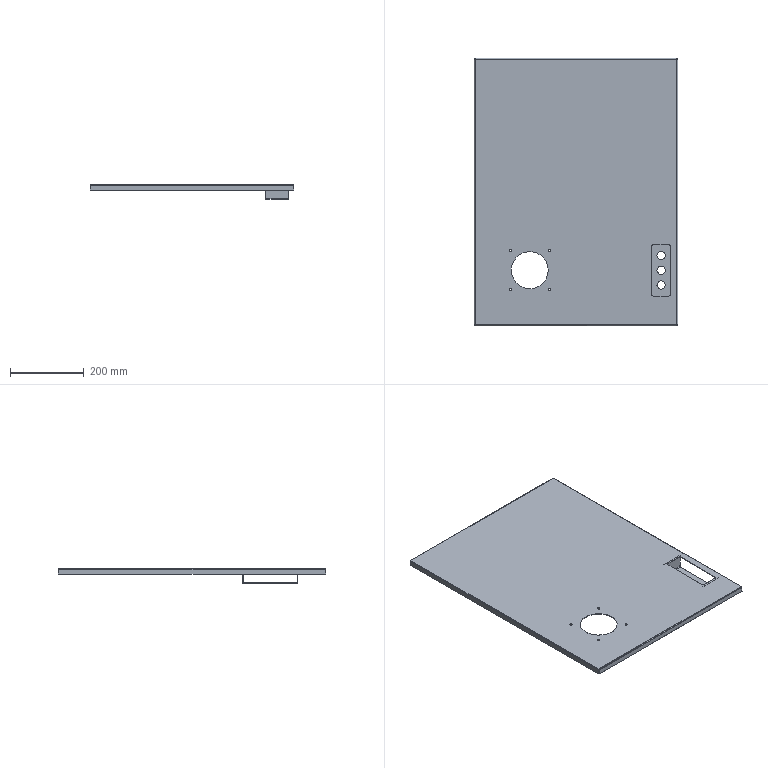Part | SolidWorks | features ICE 3, BossThin 1, FlatPattern 1, SMBaseFlange 1, SMMiteredFlange 1, SheetMetal 1 | 1 solid | 74 faces | box 550 x 723 x 40 mm | volume 641172 mm3 | plane 34 | cylinder 32 | spline 8 | commonest cylinder face diameters 6 x10 22 x6 1.473 x4 4.473 x4 10 x4 3 x2